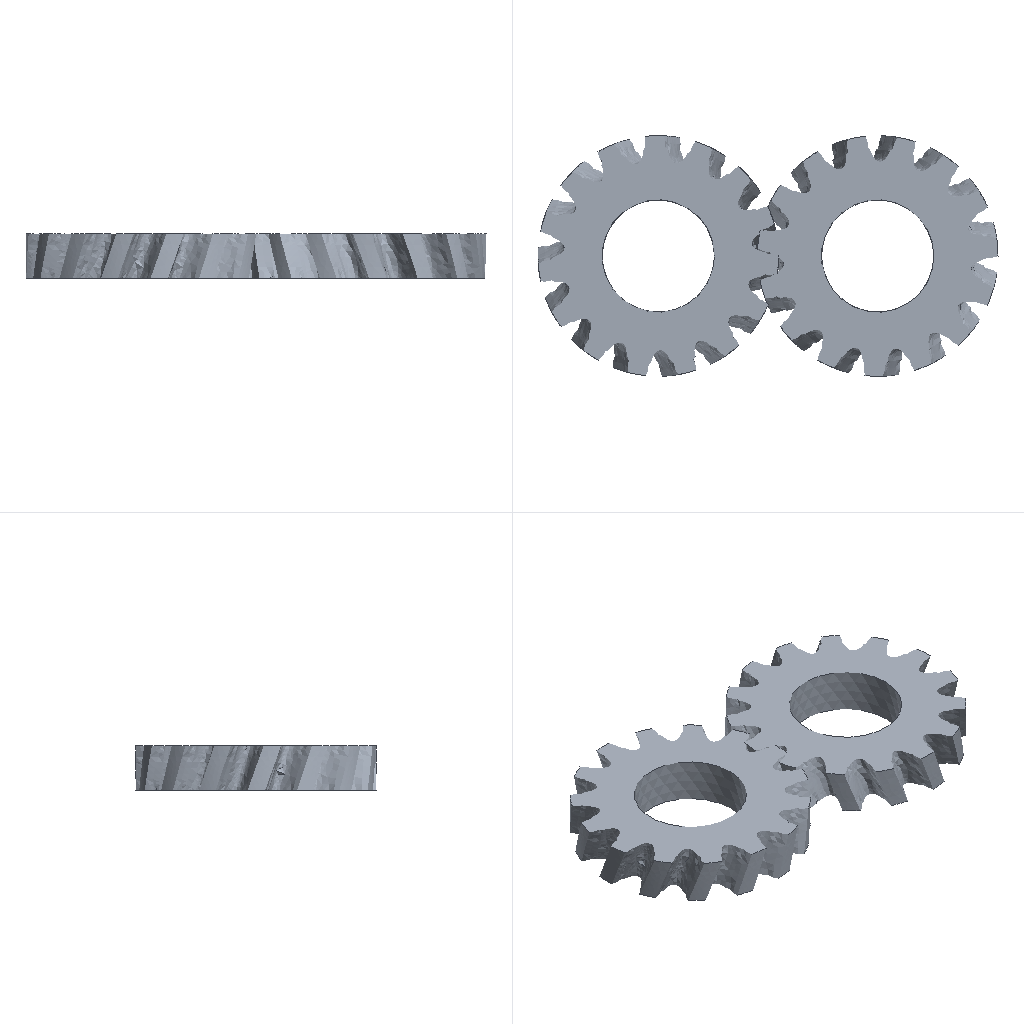Simulation study | ansys workbench
Ansys APDL input file, long lists of numbers shortened:
/batch
/config,noeldb,1     ! force off writing results to database
*get,_wallstrt,active,,time,wall
! ANSYS input file written by Workbench version 16.0 RELEASE
! File used for geometry attach: C:\Users\hmm\AppData\Local\Temp\WB_LAPTOP-92PEKBNI_hmm_19940_2\unsaved_project_files\dp0\SYS\DM\SYS.agdb
/title,yuanhu--Transient (B5)
*DIM,_wb_ProjectScratch_dir,string,248
_wb_ProjectScratch_dir(1) = 'F:\LF\self\yuanhu\WB\_ProjectScratch\ScrD866\'
*DIM,_wb_SolverFiles_dir,string,248
_wb_SolverFiles_dir(1) = 'F:\LF\self\yuanhu\WB\yuanhu_files\dp0\SYS-2\MECH\'
*DIM,_wb_userfiles_dir,string,248
_wb_userfiles_dir(1) = 'F:\LF\self\yuanhu\WB\yuanhu_files\user_files\'
/com,--- Data in consistent NMM units. See Solving Units in the help system for more information.
/units,MPA
/nopr
/wb,file,start              !  signify a WB generated input file
/prep7
! Turn off shape checking because checks already performed inside WB mesher.
! See help system for more information.
SHPP,OFF,,NOWARN
/nolist
etcon,set             ! allow ANSYS to choose best KEYOP's for 180x elements
/com,*********** Nodes for the whole assembly ***********
nblock,3
(1i9,3e20.9e3)
        1    6.183845739E+001   -1.519273240E+001    4.233906430E+000
! (51987 more lines like these left out)
-1
/wb,elem,start            !  set before creation of elements
/com,*********** Elements for Body 1 "Solid" ***********
et,1,187
eblock,19,solid,,11470
(19i9)
        1        1        1        1        0        0        0        0       10        0        1        2        8      444        9     4085     4078     4145     4116
! (22939 more lines like these left out)
-1
/com,*********** Elements for Body 2 "Solid" ***********
et,2,187
eblock,19,solid,,14800
(19i9)
        2        2        2        2        0        0        0        0       10        0    11471    23126    24680    25907    25826    28074    45158    28065    28080
! (29599 more lines like these left out)
-1
/wb,elem,end               !  done creating elements
/com,*********** Send User Defined Coordinate System(s) ***********
local,12,0,48.804,3.57140444047492e-015,5.,-0.,0.,0.
local,13,0,0.,-7.65404249467096e-016,5.,-0.,0.,0.
csys,0
toffst,273.15,  ! Temperature offset from absolute zero
/com,*********** Set Reference Temperature ***********
tref,22.
/wb,mat,start              !  starting to send materials
/com,*********** Send Materials ***********
MP,DENS,1,7.85e-09,	! tonne mm^-3
MP,ALPX,1,1.2e-05,	! C^-1
MP,C,1,434000000,	! mm^2 s^-2 C^-1
MP,KXX,1,60.5,	! tonne mm s^-3 C^-1
MP,RSVX,1,0.00017,	! ohm mm
MP,EX,1,200000,	! tonne s^-2 mm^-1
MP,NUXY,1,0.3,
MP,MURX,1,10000,
MP,DENS,2,7.85e-09,	! tonne mm^-3
MP,ALPX,2,1.2e-05,	! C^-1
MP,C,2,434000000,	! mm^2 s^-2 C^-1
MP,KXX,2,60.5,	! tonne mm s^-3 C^-1
MP,RSVX,2,0.00017,	! ohm mm
MP,EX,2,200000,	! tonne s^-2 mm^-1
MP,NUXY,2,0.3,
MP,MURX,2,10000,
/wb,mat,end                !  done sending materials
!************************* Model Summary ********************
!Solid,	Structural Steel,	matid,	1
!Solid,	Structural Steel,	matid,	2
!************************* End Model Summary ********************
! get the diagonal of the bounding box. Needed later for other things
*get,_xmin,node,,mnloc,x
*get,_ymin,node,,mnloc,y
*get,_zmin,node,,mnloc,z
*get,_xmax,node,,mxloc,x
*get,_ymax,node,,mxloc,y
*get,_zmax,node,,mxloc,z
_ASMDIAG=(_xmax-_xmin)*(_xmax-_xmin)+(_ymax-_ymin)*(_ymax-_ymin)+(_zmax-_zmin)*(_zmax-_zmin)
_ASMDIAG=SQRT(_ASMDIAG)
/wb,contact,start          !  starting to send contact
/com,*********** Create Contact "Frictional - No Selection To No Selection" ***********
/com,            Real Constant Set For Above Contact Is 4 & 3
*set,tid,4
*set,cid,3
r,tid
r,cid
et,tid,170
et,cid,174
eblock,10,,,3036
(15i9)
    26277        4        4        4        0     2495     2490     2493     2493    16197    16195     2493    16196
! (3035 more lines like these left out)
-1
eblock,10,,,3036
(15i9)
    29313        3        3        3        0     2495     2490     2493     2493    16197    16195     2493    16196
! (3035 more lines like these left out)
-1
eblock,10,,,4294
(15i9)
    32349        3        4        3        0    26571    26575    26578    26578    44256    44254    26578    44255
! (4293 more lines like these left out)
-1
eblock,10,,,4294
(15i9)
    36643        4        3        4        0    26571    26575    26578    26578    44256    44254    26578    44255
! (4293 more lines like these left out)
-1
keyo,cid,8,2               ! auto create asymmetric contact (from Program Controlled setting)
keyo,cid,10,2              ! adjust contact stiffness each NR iteration (from Program Controlled setting)
keyo,cid,12,0              ! standard contact
mp,mu,cid,0.1	! unitless
keyo,cid,2,0               ! augmented Lagrange (from Program Controlled setting)
keyo,cid,4,0               ! on Gauss point (from Program Controlled setting)
keyo,cid,9,0               ! use real geometry with stepped effects
keyo,cid,7,0               ! No Prediction
rmod,tid,3,1.	! FKN
rmod,tid,5,0.	! ICONT
rmod,tid,6,0.	! PINB
rmod,tid,10,0.	! CNOF
rmod,tid,12,0.	! FKT
rmod,tid,36,44	! WB DSID
rmod,cid,3,1.	! FKN
rmod,cid,5,0.	! ICONT
rmod,cid,6,0.	! PINB
rmod,cid,10,0.	! CNOF
rmod,cid,12,0.	! FKT
rmod,cid,36,44	! WB DSID
nsel,all
esel,all
/wb,contact,end            !  done creating contacts
/com,*********** Send Named Selection as Node Component ***********
CMBLOCK,SELECTION,NODE,     6867
(8i10)
        11        12       433       434       435       436       437       438
! (858 more lines like these left out)
/com,*********** Send Named Selection as Node Component ***********
CMBLOCK,SELECTION_2,NODE,     9383
(8i10)
     23134     23135     23141     23142     23143     23158     23169     23195
! (1172 more lines like these left out)
/golist
/wb,load,start             !  starting to send loads
nsel,all
/com,*********** Create Remote Point "Internal Remote Point 2" ***********
! -------- Remote Point Used by "Revolute - Ground To Solid" --------
*set,tid,6
*set,cid,5
et,cid,174
et,tid,170
keyo,tid,2,1               ! Don't fix the pilot node
keyo,tid,4,0               ! Activate all DOF's due to large deformation
keyo,cid,12,5              ! Bonded Contact
keyo,cid,4,2               ! Rigid CERIG style load
keyo,cid,2,2               ! MPC style contact
eblock,10,,,200
(15i9)
    40937        5        5        5        0     1337      704     1343     1343    22904    22894     1343    22901
! (199 more lines like these left out)
-1
*set,_npilot,51986
_npilot50=_npilot
type,tid
mat ,cid
real,cid
tshape,pilo
en,41137,_npilot
tshape
/com,*********** Create Remote Point "Internal Remote Point 4" ***********
! -------- Remote Point Used by "Revolute - Ground To Solid" --------
*set,tid,8
*set,cid,7
et,cid,174
et,tid,170
keyo,tid,2,1               ! Don't fix the pilot node
keyo,tid,4,0               ! Activate all DOF's due to large deformation
keyo,cid,12,5              ! Bonded Contact
keyo,cid,4,2               ! Rigid CERIG style load
keyo,cid,2,2               ! MPC style contact
eblock,10,,,200
(15i9)
    41138        7        7        7        0    24651    25201    25240    25240    51943    51513    25240    51942
! (199 more lines like these left out)
-1
*set,_npilot,51988
_npilot57=_npilot
type,tid
mat ,cid
real,cid
tshape,pilo
en,41338,_npilot
tshape
/com,*********** Create Joint "Revolute - Ground To Solid" ***********
/com,            Real Constant Set For Above Joint Is 9
! Joint Element Type Declaration and Definition using MPC184
*set,_jid,9
et,_jid,184
keyo,_jid,1,6           ! Revolute Joint
keyo,_jid,4,1           ! Z Axis is revolute axis
sectype,_jid, joint, revo, _wbjoint
secjoint,,12,12
mat,_jid
real,_jid
type,_jid
secnum,_jid
en,26273,,51986        ! body to ground joint
/com,*********** Create Joint "Revolute - Ground To Solid" ***********
/com,            Real Constant Set For Above Joint Is 10
! Joint Element Type Declaration and Definition using MPC184
*set,_jid,10
et,_jid,184
keyo,_jid,1,6           ! Revolute Joint
keyo,_jid,4,1           ! Z Axis is revolute axis
sectype,_jid, joint, revo, _wbjoint
secjoint,,13,13
mat,_jid
real,_jid
type,_jid
secnum,_jid
en,26276,,51988        ! body to ground joint
/com,*********** Create Joint Drivers **********
*DIM,_loadvari78,TABLE,3,1,1,TIME,
! Time values
_loadvari78(1,0,1) = 0.
_loadvari78(2,0,1) = 0.3
_loadvari78(3,0,1) = 2.
! Load values
_loadvari78(1,1,1) = 0.
_loadvari78(2,1,1) = 1.74532925199433e-003
_loadvari78(3,1,1) = 3.49065850398866e-002
/gst,on,on
fini
*get,_numnode,node,0,count
*get,_numelem,elem,0,count
*get, _MAXELEMNUM, elem, 0, NUM, MAX
*get, _MAXNODENUM, node, 0, NUM, MAX
*get, _MAXELEMTYPE, etyp, 0, NUM, MAX
*get, _MAXREALCONST, real, 0, NUM, MAX
/go
/wb,load,end               !  done creating loads
/com,--- Number of total nodes = %_numnode%
/com,--- Number of contact elements = 15060
/com,--- Number of spring elements = 0
/com,--- Number of bearing elements = 0
/com,--- Number of solid elements = 26270
/com,--- Number of total elements = %_numelem%
*get,_wallbsol,active,,time,wall
/com,****************************************************************************
/com,*************************    SOLUTION       ********************************
/com,****************************************************************************
/solu
antype,4                   ! transient analysis
nlgeom,on                  ! Turn on Large Deformation Effects
kbc,1                      ! stepped BC's
eqsl,pcg,1e-8,,,,,,1
cntr,print,1               ! print out contact info and also make no initial contact an error
trnopt,full,,,,,hht        ! HHT time integration method
tintp,0.1	! Numerical Damping
nldiag,cont,iter           ! print out contact info each equilibrium iteration
resc,define,last,last,,dele	   ! Program Controlled
/com,****************************************************
/com,******************* SOLVE FOR LS 1 ****************
/nopr
/gopr
esel,s,type,,9
dj,all,rotz,%_loadvari78%
esel,all
autots,on                   ! User turned on automatic time stepping
deltim,0.05,0.05,0.05,OFF
time,0.3
timint,on                  ! Turn on time integration effects
outres,erase
outres,all,none
outres,nsol,all
outres,rsol,all
outres,strs,all
outres,epel,all
outres,eppl,all
outres,v,all
outres,a,all
/nopr
esel,s,mat,,9
esel,a,mat,,10
cm,_elmisc,elem
esel,all
/gopr
outres,misc,all,_elmisc
stabilize,off                   ! Stabilization turned OFF by user
! *********** WB SOLVE COMMAND ***********
! check interactive state
*get,ANSINTER_,active,,int
*if,ANSINTER_,ne,0,then
/eof
*endif
solve
/com *************** Write FE CONNECTORS *********
CEWRITE,file,ce,,INTE
/com,****************************************************
/com,*************** FINISHED SOLVE FOR LS 1 *************
/com,****************************************************
/com,******************* SOLVE FOR LS 2 ****************
/nopr
/gopr
autots,on                   ! User turned on automatic time stepping
deltim,0.1,0.1,0.1,OFF
time,2.
timint,on                  ! Turn on time integration effects
outres,erase
outres,all,none
outres,nsol,all
outres,rsol,all
outres,strs,all
outres,epel,all
outres,eppl,all
outres,v,all
outres,a,all
outres,misc,all,_elmisc
stabilize,off                   ! Stabilization turned OFF by user
solve
/com,****************************************************
/com,*************** FINISHED SOLVE FOR LS 2 *************
*set,_DS_PROGRESS          ! turn off progress updates to avoid virus scanning bug
*get,_wallasol,active,,time,wall
/nopr
*get,_numnode,node,0,count
*get,_numelem,elem,0,count
*get, _MAXELEMNUM, elem, 0, NUM, MAX
*get, _MAXNODENUM, node, 0, NUM, MAX,,,INTERNAL
*get, _MAXELEMTYPE, etyp, 0, NUM, MAX
*get, _MAXREALCONST, real, 0, NUM, MAX
/gopr
*get,_PCGITER,active,,solu,cgiter
/post1
xmlo,ENCODING,ISO-8859-1
xmlo,parm
/xml,parm,xml
fini
/gopr
*get,_walldone,active,,time,wall
_preptime=(_wallbsol-_wallstrt)*3600
_solvtime=(_wallasol-_wallbsol)*3600
_posttime=(_walldone-_wallasol)*3600
_totaltim=(_walldone-_wallstrt)*3600
/wb,file,end               ! done with WB generated input